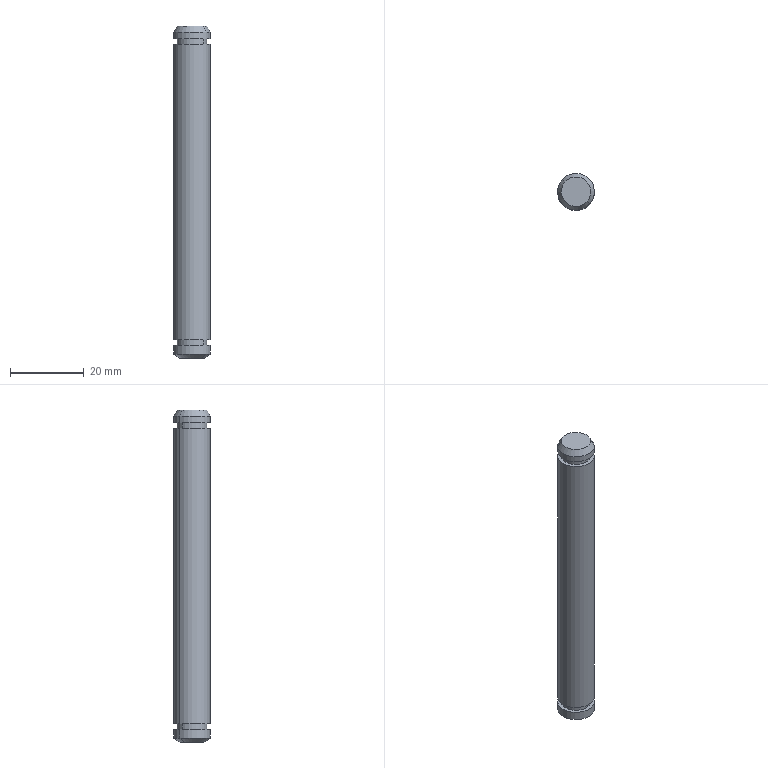Part | NX | features BREP 1 | 1 solid | 20 faces | box 10 x 10 x 90 mm | volume 6929 mm3 | cylinder 10 | plane 6 | cone 4 | commonest cylinder face diameters 10 x6 8 x4
STEP:
#1=CARTESIAN_POINT('',(29.203,158.704,45.));
#2=VERTEX_POINT('',#1);
#3=CARTESIAN_POINT('',(23.139,163.922,45.));
#4=VERTEX_POINT('',#3);
#5=CARTESIAN_POINT('',(26.171,161.313,45.));
#6=DIRECTION('',(0.,0.,1.));
#7=DIRECTION('',(0.758,-0.6522,0.));
#8=AXIS2_PLACEMENT_3D('',#5,#6,#7);
#9=CIRCLE('',#8,4.);
#10=EDGE_CURVE('',#2,#4,#9,.T.);
#11=ORIENTED_EDGE('',*,*,#10,.F.);
#12=CARTESIAN_POINT('',(29.961,158.052,43.268));
#13=VERTEX_POINT('',#12);
#14=CARTESIAN_POINT('',(29.961,158.052,43.268));
#15=DIRECTION('',(-0.379,0.3261,0.866));
#16=VECTOR('',#15,1000.);
#17=LINE('',#14,#16);
#18=EDGE_CURVE('',#13,#2,#17,.T.);
#19=ORIENTED_EDGE('',*,*,#18,.F.);
#20=CARTESIAN_POINT('',(22.381,164.574,43.268));
#21=VERTEX_POINT('',#20);
#22=CARTESIAN_POINT('',(26.171,161.313,43.268));
#23=DIRECTION('',(0.,0.,-1.));
#24=DIRECTION('',(0.758,-0.6522,0.));
#25=AXIS2_PLACEMENT_3D('',#22,#23,#24);
#26=CIRCLE('',#25,5.);
#27=EDGE_CURVE('',#21,#13,#26,.T.);
#28=ORIENTED_EDGE('',*,*,#27,.F.);
#29=CARTESIAN_POINT('',(22.381,164.574,43.268));
#30=DIRECTION('',(-0.379,0.3261,-0.866));
#31=VECTOR('',#30,1000.);
#32=LINE('',#29,#31);
#33=EDGE_CURVE('',#4,#21,#32,.T.);
#34=ORIENTED_EDGE('',*,*,#33,.F.);
#35=EDGE_LOOP('',(#11,#19,#28,#34));
#36=FACE_BOUND('',#35,.T.);
#37=CARTESIAN_POINT('',(26.171,161.313,43.268));
#38=DIRECTION('',(0.,0.,-1.));
#39=DIRECTION('',(0.758,-0.6522,0.));
#40=AXIS2_PLACEMENT_3D('',#37,#38,#39);
#41=CONICAL_SURFACE('',#40,5.,0.5236);
#42=ADVANCED_FACE('',(#36),#41,.T.);
#43=CARTESIAN_POINT('',(23.694,163.444,-45.));
#44=VERTEX_POINT('',#43);
#45=CARTESIAN_POINT('',(28.648,159.181,-45.));
#46=VERTEX_POINT('',#45);
#47=CARTESIAN_POINT('',(26.171,161.313,-45.));
#48=DIRECTION('',(0.,0.,-1.));
#49=DIRECTION('',(-0.758,0.6522,0.));
#50=AXIS2_PLACEMENT_3D('',#47,#48,#49);
#51=CIRCLE('',#50,3.268);
#52=EDGE_CURVE('',#44,#46,#51,.T.);
#53=ORIENTED_EDGE('',*,*,#52,.F.);
#54=CARTESIAN_POINT('',(22.381,164.574,-44.));
#55=VERTEX_POINT('',#54);
#56=CARTESIAN_POINT('',(23.694,163.444,-45.));
#57=DIRECTION('',(0.6565,-0.5648,-0.5));
#58=VECTOR('',#57,1000.);
#59=LINE('',#56,#58);
#60=EDGE_CURVE('',#55,#44,#59,.T.);
#61=ORIENTED_EDGE('',*,*,#60,.F.);
#62=CARTESIAN_POINT('',(29.961,158.052,-44.));
#63=VERTEX_POINT('',#62);
#64=CARTESIAN_POINT('',(26.171,161.313,-44.));
#65=DIRECTION('',(0.,0.,1.));
#66=DIRECTION('',(-0.758,0.6522,0.));
#67=AXIS2_PLACEMENT_3D('',#64,#65,#66);
#68=CIRCLE('',#67,5.);
#69=EDGE_CURVE('',#63,#55,#68,.T.);
#70=ORIENTED_EDGE('',*,*,#69,.F.);
#71=CARTESIAN_POINT('',(28.648,159.181,-45.));
#72=DIRECTION('',(0.6565,-0.5648,0.5));
#73=VECTOR('',#72,1000.);
#74=LINE('',#71,#73);
#75=EDGE_CURVE('',#46,#63,#74,.T.);
#76=ORIENTED_EDGE('',*,*,#75,.F.);
#77=EDGE_LOOP('',(#53,#61,#70,#76));
#78=FACE_BOUND('',#77,.T.);
#79=CARTESIAN_POINT('',(26.171,161.313,-45.));
#80=DIRECTION('',(0.,0.,1.));
#81=DIRECTION('',(-0.758,0.6522,0.));
#82=AXIS2_PLACEMENT_3D('',#79,#80,#81);
#83=CONICAL_SURFACE('',#82,3.268,1.047);
#84=ADVANCED_FACE('',(#78),#83,.T.);
#85=CARTESIAN_POINT('',(22.381,164.574,41.6));
#86=VERTEX_POINT('',#85);
#87=CARTESIAN_POINT('',(29.961,158.052,41.6));
#88=VERTEX_POINT('',#87);
#89=CARTESIAN_POINT('',(26.171,161.313,41.6));
#90=DIRECTION('',(0.,0.,-1.));
#91=DIRECTION('',(-0.758,0.6522,0.));
#92=AXIS2_PLACEMENT_3D('',#89,#90,#91);
#93=CIRCLE('',#92,5.);
#94=EDGE_CURVE('',#86,#88,#93,.T.);
#95=ORIENTED_EDGE('',*,*,#94,.F.);
#96=CARTESIAN_POINT('',(22.381,164.574,-45.));
#97=DIRECTION('',(0.,0.,-1.));
#98=VECTOR('',#97,1000.);
#99=LINE('',#96,#98);
#100=EDGE_CURVE('',#21,#86,#99,.T.);
#101=ORIENTED_EDGE('',*,*,#100,.F.);
#102=ORIENTED_EDGE('',*,*,#27,.T.);
#103=CARTESIAN_POINT('',(29.961,158.052,-45.));
#104=DIRECTION('',(0.,0.,1.));
#105=VECTOR('',#104,1000.);
#106=LINE('',#103,#105);
#107=EDGE_CURVE('',#88,#13,#106,.T.);
#108=ORIENTED_EDGE('',*,*,#107,.F.);
#109=EDGE_LOOP('',(#95,#101,#102,#108));
#110=FACE_BOUND('',#109,.T.);
#111=CARTESIAN_POINT('',(26.171,161.313,-45.));
#112=DIRECTION('',(0.,0.,1.));
#113=DIRECTION('',(-0.758,0.6522,0.));
#114=AXIS2_PLACEMENT_3D('',#111,#112,#113);
#115=CYLINDRICAL_SURFACE('',#114,5.);
#116=ADVANCED_FACE('',(#110),#115,.T.);
#117=CARTESIAN_POINT('',(23.139,163.922,41.6));
#118=VERTEX_POINT('',#117);
#119=CARTESIAN_POINT('',(29.203,158.704,41.6));
#120=VERTEX_POINT('',#119);
#121=CARTESIAN_POINT('',(26.171,161.313,41.6));
#122=DIRECTION('',(0.,0.,-1.));
#123=DIRECTION('',(-0.758,0.6522,0.));
#124=AXIS2_PLACEMENT_3D('',#121,#122,#123);
#125=CIRCLE('',#124,4.);
#126=EDGE_CURVE('',#118,#120,#125,.T.);
#127=ORIENTED_EDGE('',*,*,#126,.T.);
#128=CARTESIAN_POINT('',(29.203,158.704,40.));
#129=VERTEX_POINT('',#128);
#130=CARTESIAN_POINT('',(29.203,158.704,41.6));
#131=DIRECTION('',(0.,0.,-1.));
#132=VECTOR('',#131,1000.);
#133=LINE('',#130,#132);
#134=EDGE_CURVE('',#120,#129,#133,.T.);
#135=ORIENTED_EDGE('',*,*,#134,.T.);
#136=CARTESIAN_POINT('',(23.139,163.922,40.));
#137=VERTEX_POINT('',#136);
#138=CARTESIAN_POINT('',(26.171,161.313,40.));
#139=DIRECTION('',(0.,0.,-1.));
#140=DIRECTION('',(-0.758,0.6522,0.));
#141=AXIS2_PLACEMENT_3D('',#138,#139,#140);
#142=CIRCLE('',#141,4.);
#143=EDGE_CURVE('',#137,#129,#142,.T.);
#144=ORIENTED_EDGE('',*,*,#143,.F.);
#145=CARTESIAN_POINT('',(23.139,163.922,41.6));
#146=DIRECTION('',(0.,0.,1.));
#147=VECTOR('',#146,1000.);
#148=LINE('',#145,#147);
#149=EDGE_CURVE('',#137,#118,#148,.T.);
#150=ORIENTED_EDGE('',*,*,#149,.T.);
#151=EDGE_LOOP('',(#127,#135,#144,#150));
#152=FACE_BOUND('',#151,.T.);
#153=CARTESIAN_POINT('',(26.171,161.313,41.6));
#154=DIRECTION('',(0.,0.,-1.));
#155=DIRECTION('',(0.758,-0.6522,0.));
#156=AXIS2_PLACEMENT_3D('',#153,#154,#155);
#157=CYLINDRICAL_SURFACE('',#156,4.);
#158=ADVANCED_FACE('',(#152),#157,.T.);
#159=CARTESIAN_POINT('',(23.139,163.922,-41.6));
#160=VERTEX_POINT('',#159);
#161=CARTESIAN_POINT('',(29.203,158.704,-41.6));
#162=VERTEX_POINT('',#161);
#163=CARTESIAN_POINT('',(26.171,161.313,-41.6));
#164=DIRECTION('',(0.,0.,-1.));
#165=DIRECTION('',(-0.758,0.6522,0.));
#166=AXIS2_PLACEMENT_3D('',#163,#164,#165);
#167=CIRCLE('',#166,4.);
#168=EDGE_CURVE('',#160,#162,#167,.T.);
#169=ORIENTED_EDGE('',*,*,#168,.F.);
#170=CARTESIAN_POINT('',(23.139,163.922,-40.));
#171=VERTEX_POINT('',#170);
#172=CARTESIAN_POINT('',(23.139,163.922,-41.6));
#173=DIRECTION('',(0.,0.,-1.));
#174=VECTOR('',#173,1000.);
#175=LINE('',#172,#174);
#176=EDGE_CURVE('',#171,#160,#175,.T.);
#177=ORIENTED_EDGE('',*,*,#176,.F.);
#178=CARTESIAN_POINT('',(29.203,158.704,-40.));
#179=VERTEX_POINT('',#178);
#180=CARTESIAN_POINT('',(26.171,161.313,-40.));
#181=DIRECTION('',(0.,0.,-1.));
#182=DIRECTION('',(-0.758,0.6522,0.));
#183=AXIS2_PLACEMENT_3D('',#180,#181,#182);
#184=CIRCLE('',#183,4.);
#185=EDGE_CURVE('',#171,#179,#184,.T.);
#186=ORIENTED_EDGE('',*,*,#185,.T.);
#187=CARTESIAN_POINT('',(29.203,158.704,-41.6));
#188=DIRECTION('',(0.,0.,1.));
#189=VECTOR('',#188,1000.);
#190=LINE('',#187,#189);
#191=EDGE_CURVE('',#162,#179,#190,.T.);
#192=ORIENTED_EDGE('',*,*,#191,.F.);
#193=EDGE_LOOP('',(#169,#177,#186,#192));
#194=FACE_BOUND('',#193,.T.);
#195=CARTESIAN_POINT('',(26.171,161.313,-41.6));
#196=DIRECTION('',(0.,0.,1.));
#197=DIRECTION('',(-0.758,0.6522,0.));
#198=AXIS2_PLACEMENT_3D('',#195,#196,#197);
#199=CYLINDRICAL_SURFACE('',#198,4.);
#200=ADVANCED_FACE('',(#194),#199,.T.);
#201=ORIENTED_EDGE('',*,*,#69,.T.);
#202=CARTESIAN_POINT('',(22.381,164.574,-41.6));
#203=VERTEX_POINT('',#202);
#204=CARTESIAN_POINT('',(22.381,164.574,-45.));
#205=DIRECTION('',(0.,0.,-1.));
#206=VECTOR('',#205,1000.);
#207=LINE('',#204,#206);
#208=EDGE_CURVE('',#203,#55,#207,.T.);
#209=ORIENTED_EDGE('',*,*,#208,.F.);
#210=CARTESIAN_POINT('',(29.961,158.052,-41.6));
#211=VERTEX_POINT('',#210);
#212=CARTESIAN_POINT('',(26.171,161.313,-41.6));
#213=DIRECTION('',(0.,0.,-1.));
#214=DIRECTION('',(-0.758,0.6522,0.));
#215=AXIS2_PLACEMENT_3D('',#212,#213,#214);
#216=CIRCLE('',#215,5.);
#217=EDGE_CURVE('',#203,#211,#216,.T.);
#218=ORIENTED_EDGE('',*,*,#217,.T.);
#219=CARTESIAN_POINT('',(29.961,158.052,-45.));
#220=DIRECTION('',(0.,0.,1.));
#221=VECTOR('',#220,1000.);
#222=LINE('',#219,#221);
#223=EDGE_CURVE('',#63,#211,#222,.T.);
#224=ORIENTED_EDGE('',*,*,#223,.F.);
#225=EDGE_LOOP('',(#201,#209,#218,#224));
#226=FACE_BOUND('',#225,.T.);
#227=CARTESIAN_POINT('',(26.171,161.313,-45.));
#228=DIRECTION('',(0.,0.,1.));
#229=DIRECTION('',(-0.758,0.6522,0.));
#230=AXIS2_PLACEMENT_3D('',#227,#228,#229);
#231=CYLINDRICAL_SURFACE('',#230,5.);
#232=ADVANCED_FACE('',(#226),#231,.T.);
#233=CARTESIAN_POINT('',(22.381,164.574,-40.));
#234=VERTEX_POINT('',#233);
#235=CARTESIAN_POINT('',(29.961,158.052,-40.));
#236=VERTEX_POINT('',#235);
#237=CARTESIAN_POINT('',(26.171,161.313,-40.));
#238=DIRECTION('',(0.,0.,-1.));
#239=DIRECTION('',(-0.758,0.6522,0.));
#240=AXIS2_PLACEMENT_3D('',#237,#238,#239);
#241=CIRCLE('',#240,5.);
#242=EDGE_CURVE('',#234,#236,#241,.T.);
#243=ORIENTED_EDGE('',*,*,#242,.F.);
#244=CARTESIAN_POINT('',(22.381,164.574,40.));
#245=VERTEX_POINT('',#244);
#246=CARTESIAN_POINT('',(22.381,164.574,-45.));
#247=DIRECTION('',(0.,0.,-1.));
#248=VECTOR('',#247,1000.);
#249=LINE('',#246,#248);
#250=EDGE_CURVE('',#245,#234,#249,.T.);
#251=ORIENTED_EDGE('',*,*,#250,.F.);
#252=CARTESIAN_POINT('',(29.961,158.052,40.));
#253=VERTEX_POINT('',#252);
#254=CARTESIAN_POINT('',(26.171,161.313,40.));
#255=DIRECTION('',(0.,0.,-1.));
#256=DIRECTION('',(-0.758,0.6522,0.));
#257=AXIS2_PLACEMENT_3D('',#254,#255,#256);
#258=CIRCLE('',#257,5.);
#259=EDGE_CURVE('',#245,#253,#258,.T.);
#260=ORIENTED_EDGE('',*,*,#259,.T.);
#261=CARTESIAN_POINT('',(29.961,158.052,-45.));
#262=DIRECTION('',(0.,0.,1.));
#263=VECTOR('',#262,1000.);
#264=LINE('',#261,#263);
#265=EDGE_CURVE('',#236,#253,#264,.T.);
#266=ORIENTED_EDGE('',*,*,#265,.F.);
#267=EDGE_LOOP('',(#243,#251,#260,#266));
#268=FACE_BOUND('',#267,.T.);
#269=CARTESIAN_POINT('',(26.171,161.313,-45.));
#270=DIRECTION('',(0.,0.,1.));
#271=DIRECTION('',(-0.758,0.6522,0.));
#272=AXIS2_PLACEMENT_3D('',#269,#270,#271);
#273=CYLINDRICAL_SURFACE('',#272,5.);
#274=ADVANCED_FACE('',(#268),#273,.T.);
#275=ORIENTED_EDGE('',*,*,#250,.T.);
#276=CARTESIAN_POINT('',(26.171,161.313,-40.));
#277=DIRECTION('',(0.,0.,-1.));
#278=DIRECTION('',(-0.758,0.6522,0.));
#279=AXIS2_PLACEMENT_3D('',#276,#277,#278);
#280=CIRCLE('',#279,5.);
#281=EDGE_CURVE('',#236,#234,#280,.T.);
#282=ORIENTED_EDGE('',*,*,#281,.F.);
#283=ORIENTED_EDGE('',*,*,#265,.T.);
#284=CARTESIAN_POINT('',(26.171,161.313,40.));
#285=DIRECTION('',(0.,0.,-1.));
#286=DIRECTION('',(-0.758,0.6522,0.));
#287=AXIS2_PLACEMENT_3D('',#284,#285,#286);
#288=CIRCLE('',#287,5.);
#289=EDGE_CURVE('',#253,#245,#288,.T.);
#290=ORIENTED_EDGE('',*,*,#289,.T.);
#291=EDGE_LOOP('',(#275,#282,#283,#290));
#292=FACE_BOUND('',#291,.T.);
#293=CARTESIAN_POINT('',(26.171,161.313,-45.));
#294=DIRECTION('',(0.,0.,1.));
#295=DIRECTION('',(-0.758,0.6522,0.));
#296=AXIS2_PLACEMENT_3D('',#293,#294,#295);
#297=CYLINDRICAL_SURFACE('',#296,5.);
#298=ADVANCED_FACE('',(#292),#297,.T.);
#299=ORIENTED_EDGE('',*,*,#208,.T.);
#300=CARTESIAN_POINT('',(26.171,161.313,-44.));
#301=DIRECTION('',(0.,0.,1.));
#302=DIRECTION('',(-0.758,0.6522,0.));
#303=AXIS2_PLACEMENT_3D('',#300,#301,#302);
#304=CIRCLE('',#303,5.);
#305=EDGE_CURVE('',#55,#63,#304,.T.);
#306=ORIENTED_EDGE('',*,*,#305,.T.);
#307=ORIENTED_EDGE('',*,*,#223,.T.);
#308=CARTESIAN_POINT('',(26.171,161.313,-41.6));
#309=DIRECTION('',(0.,0.,-1.));
#310=DIRECTION('',(-0.758,0.6522,0.));
#311=AXIS2_PLACEMENT_3D('',#308,#309,#310);
#312=CIRCLE('',#311,5.);
#313=EDGE_CURVE('',#211,#203,#312,.T.);
#314=ORIENTED_EDGE('',*,*,#313,.T.);
#315=EDGE_LOOP('',(#299,#306,#307,#314));
#316=FACE_BOUND('',#315,.T.);
#317=CARTESIAN_POINT('',(26.171,161.313,-45.));
#318=DIRECTION('',(0.,0.,1.));
#319=DIRECTION('',(-0.758,0.6522,0.));
#320=AXIS2_PLACEMENT_3D('',#317,#318,#319);
#321=CYLINDRICAL_SURFACE('',#320,5.);
#322=ADVANCED_FACE('',(#316),#321,.T.);
#323=CARTESIAN_POINT('',(26.171,161.313,-45.));
#324=DIRECTION('',(0.,0.,-1.));
#325=DIRECTION('',(-0.758,0.6522,0.));
#326=AXIS2_PLACEMENT_3D('',#323,#324,#325);
#327=CIRCLE('',#326,3.268);
#328=EDGE_CURVE('',#46,#44,#327,.T.);
#329=ORIENTED_EDGE('',*,*,#328,.T.);
#330=ORIENTED_EDGE('',*,*,#52,.T.);
#331=EDGE_LOOP('',(#329,#330));
#332=FACE_BOUND('',#331,.T.);
#333=CARTESIAN_POINT('',(26.171,161.313,-45.));
#334=DIRECTION('',(0.,0.,-1.));
#335=DIRECTION('',(0.758,-0.6522,0.));
#336=AXIS2_PLACEMENT_3D('',#333,#334,#335);
#337=PLANE('',#336);
#338=ADVANCED_FACE('',(#332),#337,.T.);
#339=ORIENTED_EDGE('',*,*,#313,.F.);
#340=ORIENTED_EDGE('',*,*,#217,.F.);
#341=EDGE_LOOP('',(#339,#340));
#342=FACE_BOUND('',#341,.T.);
#343=CARTESIAN_POINT('',(26.171,161.313,-41.6));
#344=DIRECTION('',(0.,0.,-1.));
#345=DIRECTION('',(-0.758,0.6522,0.));
#346=AXIS2_PLACEMENT_3D('',#343,#344,#345);
#347=CIRCLE('',#346,4.);
#348=EDGE_CURVE('',#162,#160,#347,.T.);
#349=ORIENTED_EDGE('',*,*,#348,.T.);
#350=ORIENTED_EDGE('',*,*,#168,.T.);
#351=EDGE_LOOP('',(#349,#350));
#352=FACE_BOUND('',#351,.T.);
#353=CARTESIAN_POINT('',(26.171,161.313,-41.6));
#354=DIRECTION('',(0.,0.,-1.));
#355=DIRECTION('',(0.758,-0.6522,0.));
#356=AXIS2_PLACEMENT_3D('',#353,#354,#355);
#357=PLANE('',#356);
#358=ADVANCED_FACE('',(#342,#352),#357,.F.);
#359=ORIENTED_EDGE('',*,*,#281,.T.);
#360=ORIENTED_EDGE('',*,*,#242,.T.);
#361=EDGE_LOOP('',(#359,#360));
#362=FACE_BOUND('',#361,.T.);
#363=CARTESIAN_POINT('',(26.171,161.313,-40.));
#364=DIRECTION('',(0.,0.,-1.));
#365=DIRECTION('',(-0.758,0.6522,0.));
#366=AXIS2_PLACEMENT_3D('',#363,#364,#365);
#367=CIRCLE('',#366,4.);
#368=EDGE_CURVE('',#179,#171,#367,.T.);
#369=ORIENTED_EDGE('',*,*,#368,.F.);
#370=ORIENTED_EDGE('',*,*,#185,.F.);
#371=EDGE_LOOP('',(#369,#370));
#372=FACE_BOUND('',#371,.T.);
#373=CARTESIAN_POINT('',(26.171,161.313,-40.));
#374=DIRECTION('',(0.,0.,-1.));
#375=DIRECTION('',(0.758,-0.6522,0.));
#376=AXIS2_PLACEMENT_3D('',#373,#374,#375);
#377=PLANE('',#376);
#378=ADVANCED_FACE('',(#362,#372),#377,.T.);
#379=ORIENTED_EDGE('',*,*,#176,.T.);
#380=ORIENTED_EDGE('',*,*,#348,.F.);
#381=ORIENTED_EDGE('',*,*,#191,.T.);
#382=ORIENTED_EDGE('',*,*,#368,.T.);
#383=EDGE_LOOP('',(#379,#380,#381,#382));
#384=FACE_BOUND('',#383,.T.);
#385=CARTESIAN_POINT('',(26.171,161.313,-41.6));
#386=DIRECTION('',(0.,0.,1.));
#387=DIRECTION('',(-0.758,0.6522,0.));
#388=AXIS2_PLACEMENT_3D('',#385,#386,#387);
#389=CYLINDRICAL_SURFACE('',#388,4.);
#390=ADVANCED_FACE('',(#384),#389,.T.);
#391=ORIENTED_EDGE('',*,*,#126,.F.);
#392=CARTESIAN_POINT('',(26.171,161.313,41.6));
#393=DIRECTION('',(0.,0.,-1.));
#394=DIRECTION('',(-0.758,0.6522,0.));
#395=AXIS2_PLACEMENT_3D('',#392,#393,#394);
#396=CIRCLE('',#395,4.);
#397=EDGE_CURVE('',#120,#118,#396,.T.);
#398=ORIENTED_EDGE('',*,*,#397,.F.);
#399=EDGE_LOOP('',(#391,#398));
#400=FACE_BOUND('',#399,.T.);
#401=CARTESIAN_POINT('',(26.171,161.313,41.6));
#402=DIRECTION('',(0.,0.,-1.));
#403=DIRECTION('',(-0.758,0.6522,0.));
#404=AXIS2_PLACEMENT_3D('',#401,#402,#403);
#405=CIRCLE('',#404,5.);
#406=EDGE_CURVE('',#88,#86,#405,.T.);
#407=ORIENTED_EDGE('',*,*,#406,.T.);
#408=ORIENTED_EDGE('',*,*,#94,.T.);
#409=EDGE_LOOP('',(#407,#408));
#410=FACE_BOUND('',#409,.T.);
#411=CARTESIAN_POINT('',(26.171,161.313,41.6));
#412=DIRECTION('',(0.,0.,1.));
#413=DIRECTION('',(0.758,-0.6522,0.));
#414=AXIS2_PLACEMENT_3D('',#411,#412,#413);
#415=PLANE('',#414);
#416=ADVANCED_FACE('',(#400,#410),#415,.F.);
#417=ORIENTED_EDGE('',*,*,#143,.T.);
#418=CARTESIAN_POINT('',(26.171,161.313,40.));
#419=DIRECTION('',(0.,0.,-1.));
#420=DIRECTION('',(-0.758,0.6522,0.));
#421=AXIS2_PLACEMENT_3D('',#418,#419,#420);
#422=CIRCLE('',#421,4.);
#423=EDGE_CURVE('',#129,#137,#422,.T.);
#424=ORIENTED_EDGE('',*,*,#423,.T.);
#425=EDGE_LOOP('',(#417,#424));
#426=FACE_BOUND('',#425,.T.);
#427=ORIENTED_EDGE('',*,*,#289,.F.);
#428=ORIENTED_EDGE('',*,*,#259,.F.);
#429=EDGE_LOOP('',(#427,#428));
#430=FACE_BOUND('',#429,.T.);
#431=CARTESIAN_POINT('',(26.171,161.313,40.));
#432=DIRECTION('',(0.,0.,1.));
#433=DIRECTION('',(0.758,-0.6522,0.));
#434=AXIS2_PLACEMENT_3D('',#431,#432,#433);
#435=PLANE('',#434);
#436=ADVANCED_FACE('',(#426,#430),#435,.T.);
#437=ORIENTED_EDGE('',*,*,#134,.F.);
#438=ORIENTED_EDGE('',*,*,#397,.T.);
#439=ORIENTED_EDGE('',*,*,#149,.F.);
#440=ORIENTED_EDGE('',*,*,#423,.F.);
#441=EDGE_LOOP('',(#437,#438,#439,#440));
#442=FACE_BOUND('',#441,.T.);
#443=CARTESIAN_POINT('',(26.171,161.313,41.6));
#444=DIRECTION('',(0.,0.,-1.));
#445=DIRECTION('',(0.758,-0.6522,0.));
#446=AXIS2_PLACEMENT_3D('',#443,#444,#445);
#447=CYLINDRICAL_SURFACE('',#446,4.);
#448=ADVANCED_FACE('',(#442),#447,.T.);
#449=CARTESIAN_POINT('',(26.171,161.313,45.));
#450=DIRECTION('',(0.,0.,1.));
#451=DIRECTION('',(0.758,-0.6522,0.));
#452=AXIS2_PLACEMENT_3D('',#449,#450,#451);
#453=CIRCLE('',#452,4.);
#454=EDGE_CURVE('',#4,#2,#453,.T.);
#455=ORIENTED_EDGE('',*,*,#454,.T.);
#456=ORIENTED_EDGE('',*,*,#10,.T.);
#457=EDGE_LOOP('',(#455,#456));
#458=FACE_BOUND('',#457,.T.);
#459=CARTESIAN_POINT('',(26.171,161.313,45.));
#460=DIRECTION('',(0.,0.,1.));
#461=DIRECTION('',(0.758,-0.6522,0.));
#462=AXIS2_PLACEMENT_3D('',#459,#460,#461);
#463=PLANE('',#462);
#464=ADVANCED_FACE('',(#458),#463,.T.);
#465=ORIENTED_EDGE('',*,*,#100,.T.);
#466=ORIENTED_EDGE('',*,*,#406,.F.);
#467=ORIENTED_EDGE('',*,*,#107,.T.);
#468=CARTESIAN_POINT('',(26.171,161.313,43.268));
#469=DIRECTION('',(0.,0.,-1.));
#470=DIRECTION('',(0.758,-0.6522,0.));
#471=AXIS2_PLACEMENT_3D('',#468,#469,#470);
#472=CIRCLE('',#471,5.);
#473=EDGE_CURVE('',#13,#21,#472,.T.);
#474=ORIENTED_EDGE('',*,*,#473,.T.);
#475=EDGE_LOOP('',(#465,#466,#467,#474));
#476=FACE_BOUND('',#475,.T.);
#477=CARTESIAN_POINT('',(26.171,161.313,-45.));
#478=DIRECTION('',(0.,0.,1.));
#479=DIRECTION('',(-0.758,0.6522,0.));
#480=AXIS2_PLACEMENT_3D('',#477,#478,#479);
#481=CYLINDRICAL_SURFACE('',#480,5.);
#482=ADVANCED_FACE('',(#476),#481,.T.);
#483=ORIENTED_EDGE('',*,*,#60,.T.);
#484=ORIENTED_EDGE('',*,*,#328,.F.);
#485=ORIENTED_EDGE('',*,*,#75,.T.);
#486=ORIENTED_EDGE('',*,*,#305,.F.);
#487=EDGE_LOOP('',(#483,#484,#485,#486));
#488=FACE_BOUND('',#487,.T.);
#489=CARTESIAN_POINT('',(26.171,161.313,-45.));
#490=DIRECTION('',(0.,0.,1.));
#491=DIRECTION('',(-0.758,0.6522,0.));
#492=AXIS2_PLACEMENT_3D('',#489,#490,#491);
#493=CONICAL_SURFACE('',#492,3.268,1.047);
#494=ADVANCED_FACE('',(#488),#493,.T.);
#495=ORIENTED_EDGE('',*,*,#18,.T.);
#496=ORIENTED_EDGE('',*,*,#454,.F.);
#497=ORIENTED_EDGE('',*,*,#33,.T.);
#498=ORIENTED_EDGE('',*,*,#473,.F.);
#499=EDGE_LOOP('',(#495,#496,#497,#498));
#500=FACE_BOUND('',#499,.T.);
#501=CARTESIAN_POINT('',(26.171,161.313,43.268));
#502=DIRECTION('',(0.,0.,-1.));
#503=DIRECTION('',(0.758,-0.6522,0.));
#504=AXIS2_PLACEMENT_3D('',#501,#502,#503);
#505=CONICAL_SURFACE('',#504,5.,0.5236);
#506=ADVANCED_FACE('',(#500),#505,.T.);
#507=CLOSED_SHELL('',(#42,#84,#116,#158,#200,#232,#274,#298,#322,#338,#358,#378,#390,#416,#436,#448,#464,#482,#494,#506));
#508=MANIFOLD_SOLID_BREP('',#507);
#509=(LENGTH_UNIT()NAMED_UNIT(*)SI_UNIT(.MILLI.,.METRE.));
#510=UNCERTAINTY_MEASURE_WITH_UNIT(LENGTH_MEASURE(0.00001),#509,'','');
#511=(NAMED_UNIT(*)PLANE_ANGLE_UNIT()SI_UNIT($,.RADIAN.));
#512=(NAMED_UNIT(*)SI_UNIT($,.STERADIAN.)SOLID_ANGLE_UNIT());
#513=(GEOMETRIC_REPRESENTATION_CONTEXT(3)GLOBAL_UNCERTAINTY_ASSIGNED_CONTEXT((#510))GLOBAL_UNIT_ASSIGNED_CONTEXT((#509,#511,#512))REPRESENTATION_CONTEXT('',''));
#514=ADVANCED_BREP_SHAPE_REPRESENTATION('',(#508),#513);